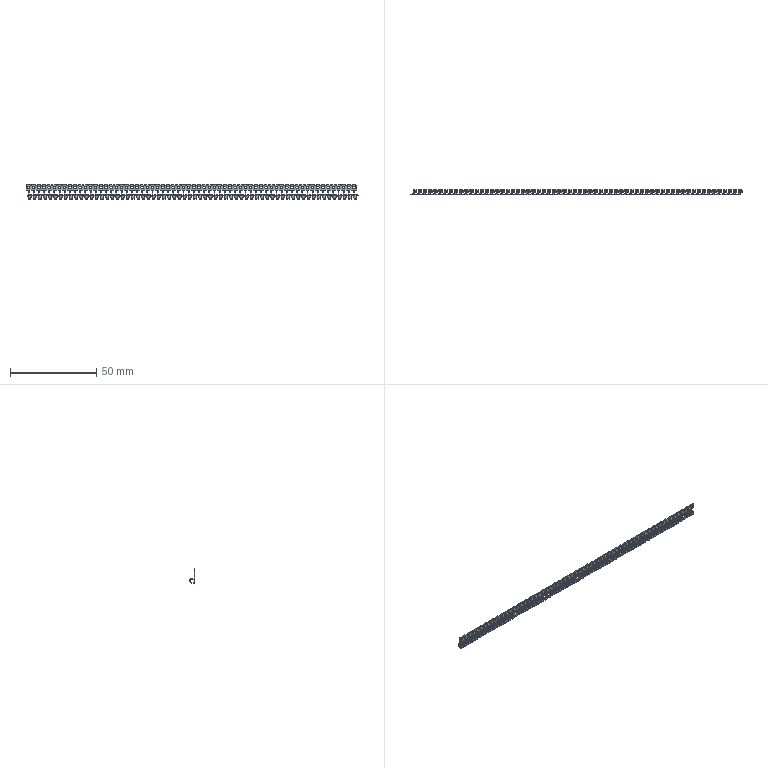Part | NX | 1 solid | 7174 faces | volume 253.143 mm3 | plane 3078 | cylinder 2560 | torus 1280 | sphere 256 | commonest cylinder face diameters 0.2 x512 0.8 x320 0.12 x256 0.4 x256 0.44 x256 0.52 x256